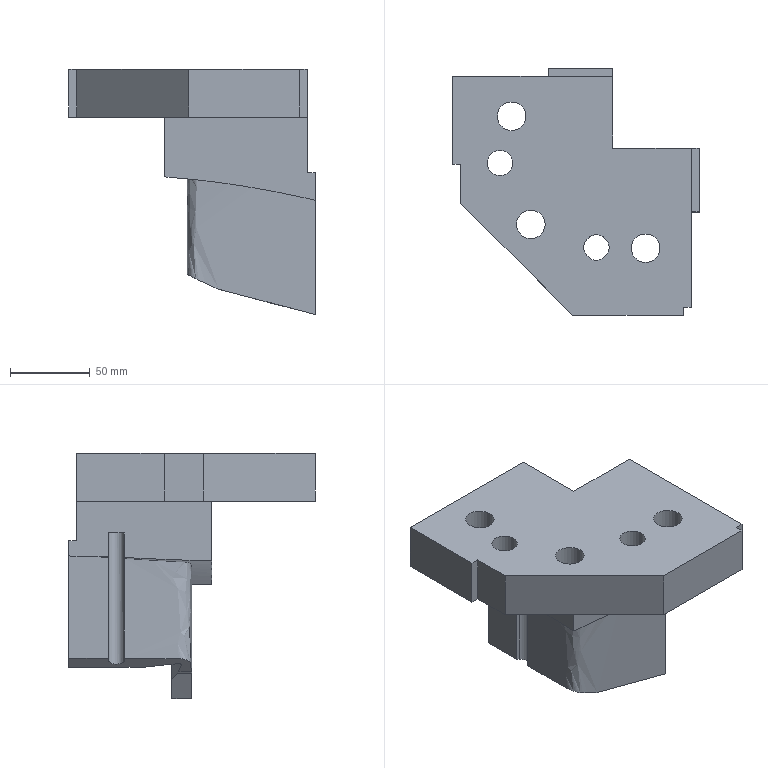Part | NX | features solid 2 | 1 solid | 43 faces | box 155 x 155 x 154.045 mm | volume 824423 mm3 | plane 23 | spline 11 | cylinder 9 | commonest cylinder face diameters 18 x3 26 x3 16 x2 10 x1